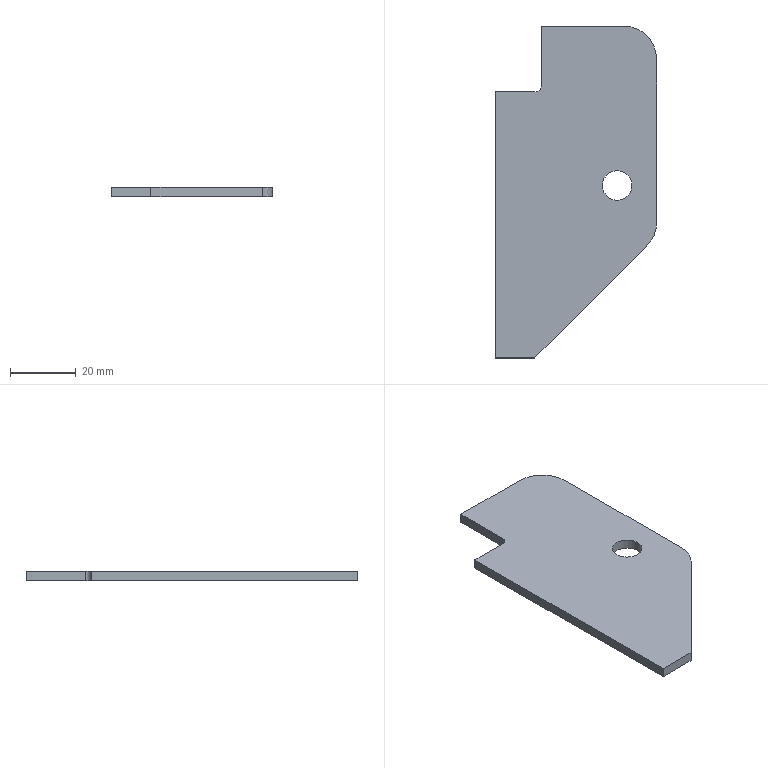Part | STEP file | 750038332 | 1 solid | 14 faces | box 49 x 101 x 3 mm | volume 11694 mm3 | plane 9 | cylinder 5 | commonest cylinder face diameters 9 x2 20 x2 4 x1
STEP:
#1=CARTESIAN_POINT('',(32.5,52.5,3.));
#2=VERTEX_POINT('',#1);
#3=CARTESIAN_POINT('',(41.5,52.5,3.));
#4=VERTEX_POINT('',#3);
#5=CARTESIAN_POINT('',(37.,52.5,3.));
#6=DIRECTION('',(0.,0.,1.));
#7=DIRECTION('',(-1.,0.,0.));
#8=AXIS2_PLACEMENT_3D('',#5,#6,#7);
#9=CIRCLE('',#8,4.5);
#10=EDGE_CURVE('',#2,#4,#9,.T.);
#11=ORIENTED_EDGE('',*,*,#10,.T.);
#12=CARTESIAN_POINT('',(41.5,52.5,0.));
#13=VERTEX_POINT('',#12);
#14=CARTESIAN_POINT('',(41.5,52.5,3.));
#15=DIRECTION('',(0.,0.,-1.));
#16=VECTOR('',#15,1000.);
#17=LINE('',#14,#16);
#18=EDGE_CURVE('',#4,#13,#17,.T.);
#19=ORIENTED_EDGE('',*,*,#18,.T.);
#20=CARTESIAN_POINT('',(32.5,52.5,0.));
#21=VERTEX_POINT('',#20);
#22=CARTESIAN_POINT('',(37.,52.5,0.));
#23=DIRECTION('',(0.,0.,1.));
#24=DIRECTION('',(-1.,0.,0.));
#25=AXIS2_PLACEMENT_3D('',#22,#23,#24);
#26=CIRCLE('',#25,4.5);
#27=EDGE_CURVE('',#21,#13,#26,.T.);
#28=ORIENTED_EDGE('',*,*,#27,.F.);
#29=CARTESIAN_POINT('',(32.5,52.5,3.));
#30=DIRECTION('',(0.,0.,-1.));
#31=VECTOR('',#30,1000.);
#32=LINE('',#29,#31);
#33=EDGE_CURVE('',#2,#21,#32,.T.);
#34=ORIENTED_EDGE('',*,*,#33,.F.);
#35=EDGE_LOOP('',(#11,#19,#28,#34));
#36=FACE_OUTER_BOUND('',#35,.T.);
#37=CARTESIAN_POINT('',(37.,52.5,3.));
#38=DIRECTION('',(0.,0.,-1.));
#39=DIRECTION('',(-1.,0.,0.));
#40=AXIS2_PLACEMENT_3D('',#37,#38,#39);
#41=CYLINDRICAL_SURFACE('',#40,4.5);
#42=ADVANCED_FACE('',(#36),#41,.F.);
#43=ORIENTED_EDGE('',*,*,#10,.F.);
#44=CARTESIAN_POINT('',(37.,52.5,3.));
#45=DIRECTION('',(0.,0.,1.));
#46=DIRECTION('',(-1.,0.,0.));
#47=AXIS2_PLACEMENT_3D('',#44,#45,#46);
#48=CIRCLE('',#47,4.5);
#49=EDGE_CURVE('',#4,#2,#48,.T.);
#50=ORIENTED_EDGE('',*,*,#49,.F.);
#51=EDGE_LOOP('',(#43,#50));
#52=FACE_BOUND('',#51,.T.);
#53=CARTESIAN_POINT('',(39.,101.,3.));
#54=VERTEX_POINT('',#53);
#55=CARTESIAN_POINT('',(49.,91.,3.));
#56=VERTEX_POINT('',#55);
#57=CARTESIAN_POINT('',(39.,91.,3.));
#58=DIRECTION('',(0.,0.,-1.));
#59=DIRECTION('',(-1.,0.,0.));
#60=AXIS2_PLACEMENT_3D('',#57,#58,#59);
#61=CIRCLE('',#60,10.);
#62=EDGE_CURVE('',#54,#56,#61,.T.);
#63=ORIENTED_EDGE('',*,*,#62,.F.);
#64=CARTESIAN_POINT('',(14.,101.,3.));
#65=VERTEX_POINT('',#64);
#66=CARTESIAN_POINT('',(0.,101.,3.));
#67=DIRECTION('',(1.,0.,0.));
#68=VECTOR('',#67,1000.);
#69=LINE('',#66,#68);
#70=EDGE_CURVE('',#65,#54,#69,.T.);
#71=ORIENTED_EDGE('',*,*,#70,.F.);
#72=CARTESIAN_POINT('',(14.,83.,3.));
#73=VERTEX_POINT('',#72);
#74=CARTESIAN_POINT('',(14.,0.,3.));
#75=DIRECTION('',(0.,1.,0.));
#76=VECTOR('',#75,1000.);
#77=LINE('',#74,#76);
#78=EDGE_CURVE('',#73,#65,#77,.T.);
#79=ORIENTED_EDGE('',*,*,#78,.F.);
#80=CARTESIAN_POINT('',(12.,81.,3.));
#81=VERTEX_POINT('',#80);
#82=CARTESIAN_POINT('',(12.,83.,3.));
#83=DIRECTION('',(0.,0.,1.));
#84=DIRECTION('',(1.,0.,0.));
#85=AXIS2_PLACEMENT_3D('',#82,#83,#84);
#86=CIRCLE('',#85,2.);
#87=EDGE_CURVE('',#81,#73,#86,.T.);
#88=ORIENTED_EDGE('',*,*,#87,.F.);
#89=CARTESIAN_POINT('',(0.,81.,3.));
#90=VERTEX_POINT('',#89);
#91=CARTESIAN_POINT('',(0.,81.,3.));
#92=DIRECTION('',(1.,0.,0.));
#93=VECTOR('',#92,1000.);
#94=LINE('',#91,#93);
#95=EDGE_CURVE('',#90,#81,#94,.T.);
#96=ORIENTED_EDGE('',*,*,#95,.F.);
#97=CARTESIAN_POINT('',(0.,0.,3.));
#98=VERTEX_POINT('',#97);
#99=CARTESIAN_POINT('',(0.,0.,3.));
#100=DIRECTION('',(0.,1.,0.));
#101=VECTOR('',#100,1000.);
#102=LINE('',#99,#101);
#103=EDGE_CURVE('',#98,#90,#102,.T.);
#104=ORIENTED_EDGE('',*,*,#103,.F.);
#105=CARTESIAN_POINT('',(12.,0.,3.));
#106=VERTEX_POINT('',#105);
#107=CARTESIAN_POINT('',(0.,0.,3.));
#108=DIRECTION('',(-1.,0.,0.));
#109=VECTOR('',#108,1000.);
#110=LINE('',#107,#109);
#111=EDGE_CURVE('',#106,#98,#110,.T.);
#112=ORIENTED_EDGE('',*,*,#111,.F.);
#113=CARTESIAN_POINT('',(46.071,34.071,3.));
#114=VERTEX_POINT('',#113);
#115=CARTESIAN_POINT('',(46.071,34.071,3.));
#116=DIRECTION('',(-0.7071,-0.7071,0.));
#117=VECTOR('',#116,1000.);
#118=LINE('',#115,#117);
#119=EDGE_CURVE('',#114,#106,#118,.T.);
#120=ORIENTED_EDGE('',*,*,#119,.F.);
#121=CARTESIAN_POINT('',(49.,41.142,3.));
#122=VERTEX_POINT('',#121);
#123=CARTESIAN_POINT('',(39.,41.142,3.));
#124=DIRECTION('',(0.,0.,-1.));
#125=DIRECTION('',(-1.,0.,0.));
#126=AXIS2_PLACEMENT_3D('',#123,#124,#125);
#127=CIRCLE('',#126,10.);
#128=EDGE_CURVE('',#122,#114,#127,.T.);
#129=ORIENTED_EDGE('',*,*,#128,.F.);
#130=CARTESIAN_POINT('',(49.,0.,3.));
#131=DIRECTION('',(0.,-1.,0.));
#132=VECTOR('',#131,1000.);
#133=LINE('',#130,#132);
#134=EDGE_CURVE('',#56,#122,#133,.T.);
#135=ORIENTED_EDGE('',*,*,#134,.F.);
#136=EDGE_LOOP('',(#63,#71,#79,#88,#96,#104,#112,#120,#129,#135));
#137=FACE_OUTER_BOUND('',#136,.T.);
#138=CARTESIAN_POINT('',(0.,0.,3.));
#139=DIRECTION('',(0.,0.,-1.));
#140=DIRECTION('',(-1.,0.,0.));
#141=AXIS2_PLACEMENT_3D('',#138,#139,#140);
#142=PLANE('',#141);
#143=ADVANCED_FACE('',(#52,#137),#142,.F.);
#144=ORIENTED_EDGE('',*,*,#18,.F.);
#145=ORIENTED_EDGE('',*,*,#49,.T.);
#146=ORIENTED_EDGE('',*,*,#33,.T.);
#147=CARTESIAN_POINT('',(37.,52.5,0.));
#148=DIRECTION('',(0.,0.,1.));
#149=DIRECTION('',(-1.,0.,0.));
#150=AXIS2_PLACEMENT_3D('',#147,#148,#149);
#151=CIRCLE('',#150,4.5);
#152=EDGE_CURVE('',#13,#21,#151,.T.);
#153=ORIENTED_EDGE('',*,*,#152,.F.);
#154=EDGE_LOOP('',(#144,#145,#146,#153));
#155=FACE_OUTER_BOUND('',#154,.T.);
#156=CARTESIAN_POINT('',(37.,52.5,3.));
#157=DIRECTION('',(0.,0.,-1.));
#158=DIRECTION('',(-1.,0.,0.));
#159=AXIS2_PLACEMENT_3D('',#156,#157,#158);
#160=CYLINDRICAL_SURFACE('',#159,4.5);
#161=ADVANCED_FACE('',(#155),#160,.F.);
#162=ORIENTED_EDGE('',*,*,#134,.T.);
#163=CARTESIAN_POINT('',(49.,41.142,0.));
#164=VERTEX_POINT('',#163);
#165=CARTESIAN_POINT('',(49.,41.142,3.));
#166=DIRECTION('',(0.,0.,-1.));
#167=VECTOR('',#166,1000.);
#168=LINE('',#165,#167);
#169=EDGE_CURVE('',#122,#164,#168,.T.);
#170=ORIENTED_EDGE('',*,*,#169,.T.);
#171=CARTESIAN_POINT('',(49.,91.,0.));
#172=VERTEX_POINT('',#171);
#173=CARTESIAN_POINT('',(49.,101.,0.));
#174=DIRECTION('',(0.,1.,0.));
#175=VECTOR('',#174,1000.);
#176=LINE('',#173,#175);
#177=EDGE_CURVE('',#164,#172,#176,.T.);
#178=ORIENTED_EDGE('',*,*,#177,.T.);
#179=CARTESIAN_POINT('',(49.,91.,3.));
#180=DIRECTION('',(0.,0.,1.));
#181=VECTOR('',#180,1000.);
#182=LINE('',#179,#181);
#183=EDGE_CURVE('',#172,#56,#182,.T.);
#184=ORIENTED_EDGE('',*,*,#183,.T.);
#185=EDGE_LOOP('',(#162,#170,#178,#184));
#186=FACE_OUTER_BOUND('',#185,.T.);
#187=CARTESIAN_POINT('',(49.,101.,3.));
#188=DIRECTION('',(1.,0.,0.));
#189=DIRECTION('',(0.,1.,0.));
#190=AXIS2_PLACEMENT_3D('',#187,#188,#189);
#191=PLANE('',#190);
#192=ADVANCED_FACE('',(#186),#191,.T.);
#193=CARTESIAN_POINT('',(39.,101.,0.));
#194=VERTEX_POINT('',#193);
#195=CARTESIAN_POINT('',(39.,91.,0.));
#196=DIRECTION('',(0.,0.,1.));
#197=DIRECTION('',(-1.,0.,0.));
#198=AXIS2_PLACEMENT_3D('',#195,#196,#197);
#199=CIRCLE('',#198,10.);
#200=EDGE_CURVE('',#172,#194,#199,.T.);
#201=ORIENTED_EDGE('',*,*,#200,.T.);
#202=CARTESIAN_POINT('',(39.,101.,3.));
#203=DIRECTION('',(0.,0.,1.));
#204=VECTOR('',#203,1000.);
#205=LINE('',#202,#204);
#206=EDGE_CURVE('',#194,#54,#205,.T.);
#207=ORIENTED_EDGE('',*,*,#206,.T.);
#208=ORIENTED_EDGE('',*,*,#62,.T.);
#209=ORIENTED_EDGE('',*,*,#183,.F.);
#210=EDGE_LOOP('',(#201,#207,#208,#209));
#211=FACE_OUTER_BOUND('',#210,.T.);
#212=CARTESIAN_POINT('',(39.,91.,3.));
#213=DIRECTION('',(0.,0.,-1.));
#214=DIRECTION('',(-1.,0.,0.));
#215=AXIS2_PLACEMENT_3D('',#212,#213,#214);
#216=CYLINDRICAL_SURFACE('',#215,10.);
#217=ADVANCED_FACE('',(#211),#216,.T.);
#218=CARTESIAN_POINT('',(14.,101.,0.));
#219=VERTEX_POINT('',#218);
#220=CARTESIAN_POINT('',(14.,101.,0.));
#221=DIRECTION('',(-1.,0.,0.));
#222=VECTOR('',#221,1000.);
#223=LINE('',#220,#222);
#224=EDGE_CURVE('',#194,#219,#223,.T.);
#225=ORIENTED_EDGE('',*,*,#224,.T.);
#226=CARTESIAN_POINT('',(14.,101.,3.));
#227=DIRECTION('',(0.,0.,1.));
#228=VECTOR('',#227,1000.);
#229=LINE('',#226,#228);
#230=EDGE_CURVE('',#219,#65,#229,.T.);
#231=ORIENTED_EDGE('',*,*,#230,.T.);
#232=ORIENTED_EDGE('',*,*,#70,.T.);
#233=ORIENTED_EDGE('',*,*,#206,.F.);
#234=EDGE_LOOP('',(#225,#231,#232,#233));
#235=FACE_OUTER_BOUND('',#234,.T.);
#236=CARTESIAN_POINT('',(14.,101.,3.));
#237=DIRECTION('',(0.,1.,0.));
#238=DIRECTION('',(0.,0.,1.));
#239=AXIS2_PLACEMENT_3D('',#236,#237,#238);
#240=PLANE('',#239);
#241=ADVANCED_FACE('',(#235),#240,.T.);
#242=ORIENTED_EDGE('',*,*,#78,.T.);
#243=ORIENTED_EDGE('',*,*,#230,.F.);
#244=CARTESIAN_POINT('',(14.,83.,0.));
#245=VERTEX_POINT('',#244);
#246=CARTESIAN_POINT('',(14.,81.,0.));
#247=DIRECTION('',(0.,-1.,0.));
#248=VECTOR('',#247,1000.);
#249=LINE('',#246,#248);
#250=EDGE_CURVE('',#219,#245,#249,.T.);
#251=ORIENTED_EDGE('',*,*,#250,.T.);
#252=CARTESIAN_POINT('',(14.,83.,3.));
#253=DIRECTION('',(0.,0.,1.));
#254=VECTOR('',#253,1000.);
#255=LINE('',#252,#254);
#256=EDGE_CURVE('',#245,#73,#255,.T.);
#257=ORIENTED_EDGE('',*,*,#256,.T.);
#258=EDGE_LOOP('',(#242,#243,#251,#257));
#259=FACE_OUTER_BOUND('',#258,.T.);
#260=CARTESIAN_POINT('',(14.,81.,3.));
#261=DIRECTION('',(-1.,0.,0.));
#262=DIRECTION('',(0.,-1.,0.));
#263=AXIS2_PLACEMENT_3D('',#260,#261,#262);
#264=PLANE('',#263);
#265=ADVANCED_FACE('',(#259),#264,.T.);
#266=ORIENTED_EDGE('',*,*,#256,.F.);
#267=CARTESIAN_POINT('',(12.,81.,0.));
#268=VERTEX_POINT('',#267);
#269=CARTESIAN_POINT('',(12.,83.,0.));
#270=DIRECTION('',(0.,0.,1.));
#271=DIRECTION('',(1.,0.,0.));
#272=AXIS2_PLACEMENT_3D('',#269,#270,#271);
#273=CIRCLE('',#272,2.);
#274=EDGE_CURVE('',#268,#245,#273,.T.);
#275=ORIENTED_EDGE('',*,*,#274,.F.);
#276=CARTESIAN_POINT('',(12.,81.,3.));
#277=DIRECTION('',(0.,0.,-1.));
#278=VECTOR('',#277,1000.);
#279=LINE('',#276,#278);
#280=EDGE_CURVE('',#81,#268,#279,.T.);
#281=ORIENTED_EDGE('',*,*,#280,.F.);
#282=ORIENTED_EDGE('',*,*,#87,.T.);
#283=EDGE_LOOP('',(#266,#275,#281,#282));
#284=FACE_OUTER_BOUND('',#283,.T.);
#285=CARTESIAN_POINT('',(12.,83.,3.));
#286=DIRECTION('',(0.,0.,1.));
#287=DIRECTION('',(1.,0.,0.));
#288=AXIS2_PLACEMENT_3D('',#285,#286,#287);
#289=CYLINDRICAL_SURFACE('',#288,2.);
#290=ADVANCED_FACE('',(#284),#289,.F.);
#291=CARTESIAN_POINT('',(0.,81.,0.));
#292=VERTEX_POINT('',#291);
#293=CARTESIAN_POINT('',(0.,81.,0.));
#294=DIRECTION('',(-1.,0.,0.));
#295=VECTOR('',#294,1000.);
#296=LINE('',#293,#295);
#297=EDGE_CURVE('',#268,#292,#296,.T.);
#298=ORIENTED_EDGE('',*,*,#297,.T.);
#299=CARTESIAN_POINT('',(0.,81.,3.));
#300=DIRECTION('',(0.,0.,1.));
#301=VECTOR('',#300,1000.);
#302=LINE('',#299,#301);
#303=EDGE_CURVE('',#292,#90,#302,.T.);
#304=ORIENTED_EDGE('',*,*,#303,.T.);
#305=ORIENTED_EDGE('',*,*,#95,.T.);
#306=ORIENTED_EDGE('',*,*,#280,.T.);
#307=EDGE_LOOP('',(#298,#304,#305,#306));
#308=FACE_OUTER_BOUND('',#307,.T.);
#309=CARTESIAN_POINT('',(0.,81.,3.));
#310=DIRECTION('',(0.,1.,0.));
#311=DIRECTION('',(0.,0.,1.));
#312=AXIS2_PLACEMENT_3D('',#309,#310,#311);
#313=PLANE('',#312);
#314=ADVANCED_FACE('',(#308),#313,.T.);
#315=ORIENTED_EDGE('',*,*,#103,.T.);
#316=ORIENTED_EDGE('',*,*,#303,.F.);
#317=CARTESIAN_POINT('',(0.,0.,0.));
#318=VERTEX_POINT('',#317);
#319=CARTESIAN_POINT('',(0.,0.,0.));
#320=DIRECTION('',(0.,-1.,0.));
#321=VECTOR('',#320,1000.);
#322=LINE('',#319,#321);
#323=EDGE_CURVE('',#292,#318,#322,.T.);
#324=ORIENTED_EDGE('',*,*,#323,.T.);
#325=CARTESIAN_POINT('',(0.,0.,3.));
#326=DIRECTION('',(0.,0.,1.));
#327=VECTOR('',#326,1000.);
#328=LINE('',#325,#327);
#329=EDGE_CURVE('',#318,#98,#328,.T.);
#330=ORIENTED_EDGE('',*,*,#329,.T.);
#331=EDGE_LOOP('',(#315,#316,#324,#330));
#332=FACE_OUTER_BOUND('',#331,.T.);
#333=CARTESIAN_POINT('',(0.,0.,3.));
#334=DIRECTION('',(-1.,0.,0.));
#335=DIRECTION('',(0.,0.,1.));
#336=AXIS2_PLACEMENT_3D('',#333,#334,#335);
#337=PLANE('',#336);
#338=ADVANCED_FACE('',(#332),#337,.T.);
#339=ORIENTED_EDGE('',*,*,#111,.T.);
#340=ORIENTED_EDGE('',*,*,#329,.F.);
#341=CARTESIAN_POINT('',(12.,0.,0.));
#342=VERTEX_POINT('',#341);
#343=CARTESIAN_POINT('',(12.,0.,0.));
#344=DIRECTION('',(1.,0.,0.));
#345=VECTOR('',#344,1000.);
#346=LINE('',#343,#345);
#347=EDGE_CURVE('',#318,#342,#346,.T.);
#348=ORIENTED_EDGE('',*,*,#347,.T.);
#349=CARTESIAN_POINT('',(12.,0.,3.));
#350=DIRECTION('',(0.,0.,1.));
#351=VECTOR('',#350,1000.);
#352=LINE('',#349,#351);
#353=EDGE_CURVE('',#342,#106,#352,.T.);
#354=ORIENTED_EDGE('',*,*,#353,.T.);
#355=EDGE_LOOP('',(#339,#340,#348,#354));
#356=FACE_OUTER_BOUND('',#355,.T.);
#357=CARTESIAN_POINT('',(12.,0.,3.));
#358=DIRECTION('',(0.,-1.,0.));
#359=DIRECTION('',(0.,0.,-1.));
#360=AXIS2_PLACEMENT_3D('',#357,#358,#359);
#361=PLANE('',#360);
#362=ADVANCED_FACE('',(#356),#361,.T.);
#363=ORIENTED_EDGE('',*,*,#119,.T.);
#364=ORIENTED_EDGE('',*,*,#353,.F.);
#365=CARTESIAN_POINT('',(46.071,34.071,0.));
#366=VERTEX_POINT('',#365);
#367=CARTESIAN_POINT('',(49.,37.,0.));
#368=DIRECTION('',(0.7071,0.7071,0.));
#369=VECTOR('',#368,1000.);
#370=LINE('',#367,#369);
#371=EDGE_CURVE('',#342,#366,#370,.T.);
#372=ORIENTED_EDGE('',*,*,#371,.T.);
#373=CARTESIAN_POINT('',(46.071,34.071,3.));
#374=DIRECTION('',(0.,0.,1.));
#375=VECTOR('',#374,1000.);
#376=LINE('',#373,#375);
#377=EDGE_CURVE('',#366,#114,#376,.T.);
#378=ORIENTED_EDGE('',*,*,#377,.T.);
#379=EDGE_LOOP('',(#363,#364,#372,#378));
#380=FACE_OUTER_BOUND('',#379,.T.);
#381=CARTESIAN_POINT('',(49.,37.,3.));
#382=DIRECTION('',(0.7071,-0.7071,0.));
#383=DIRECTION('',(0.7071,0.7071,0.));
#384=AXIS2_PLACEMENT_3D('',#381,#382,#383);
#385=PLANE('',#384);
#386=ADVANCED_FACE('',(#380),#385,.T.);
#387=CARTESIAN_POINT('',(39.,41.142,0.));
#388=DIRECTION('',(0.,0.,1.));
#389=DIRECTION('',(-1.,0.,0.));
#390=AXIS2_PLACEMENT_3D('',#387,#388,#389);
#391=CIRCLE('',#390,10.);
#392=EDGE_CURVE('',#366,#164,#391,.T.);
#393=ORIENTED_EDGE('',*,*,#392,.T.);
#394=ORIENTED_EDGE('',*,*,#169,.F.);
#395=ORIENTED_EDGE('',*,*,#128,.T.);
#396=ORIENTED_EDGE('',*,*,#377,.F.);
#397=EDGE_LOOP('',(#393,#394,#395,#396));
#398=FACE_OUTER_BOUND('',#397,.T.);
#399=CARTESIAN_POINT('',(39.,41.142,3.));
#400=DIRECTION('',(0.,0.,-1.));
#401=DIRECTION('',(-1.,0.,0.));
#402=AXIS2_PLACEMENT_3D('',#399,#400,#401);
#403=CYLINDRICAL_SURFACE('',#402,10.);
#404=ADVANCED_FACE('',(#398),#403,.T.);
#405=ORIENTED_EDGE('',*,*,#27,.T.);
#406=ORIENTED_EDGE('',*,*,#152,.T.);
#407=EDGE_LOOP('',(#405,#406));
#408=FACE_BOUND('',#407,.T.);
#409=ORIENTED_EDGE('',*,*,#274,.T.);
#410=ORIENTED_EDGE('',*,*,#250,.F.);
#411=ORIENTED_EDGE('',*,*,#224,.F.);
#412=ORIENTED_EDGE('',*,*,#200,.F.);
#413=ORIENTED_EDGE('',*,*,#177,.F.);
#414=ORIENTED_EDGE('',*,*,#392,.F.);
#415=ORIENTED_EDGE('',*,*,#371,.F.);
#416=ORIENTED_EDGE('',*,*,#347,.F.);
#417=ORIENTED_EDGE('',*,*,#323,.F.);
#418=ORIENTED_EDGE('',*,*,#297,.F.);
#419=EDGE_LOOP('',(#409,#410,#411,#412,#413,#414,#415,#416,#417,#418));
#420=FACE_OUTER_BOUND('',#419,.T.);
#421=CARTESIAN_POINT('',(0.,0.,0.));
#422=DIRECTION('',(0.,0.,-1.));
#423=DIRECTION('',(-1.,0.,0.));
#424=AXIS2_PLACEMENT_3D('',#421,#422,#423);
#425=PLANE('',#424);
#426=ADVANCED_FACE('',(#408,#420),#425,.T.);
#427=CLOSED_SHELL('',(#42,#143,#161,#192,#217,#241,#265,#290,#314,#338,#362,#386,#404,#426));
#428=MANIFOLD_SOLID_BREP('',#427);
#429=CARTESIAN_POINT('',(0.,0.,0.));
#430=DIRECTION('',(0.,0.,1.));
#431=DIRECTION('',(1.,0.,0.));
#432=AXIS2_PLACEMENT_3D('',#429,#430,#431);
#433=(LENGTH_UNIT()NAMED_UNIT(*)SI_UNIT(.MILLI.,.METRE.));
#434=UNCERTAINTY_MEASURE_WITH_UNIT(LENGTH_MEASURE(0.00001),#433,'','');
#435=(NAMED_UNIT(*)PLANE_ANGLE_UNIT()SI_UNIT($,.RADIAN.));
#436=(NAMED_UNIT(*)SI_UNIT($,.STERADIAN.)SOLID_ANGLE_UNIT());
#437=(GEOMETRIC_REPRESENTATION_CONTEXT(3)GLOBAL_UNCERTAINTY_ASSIGNED_CONTEXT((#434))GLOBAL_UNIT_ASSIGNED_CONTEXT((#433,#435,#436))REPRESENTATION_CONTEXT('',''));
#438=ADVANCED_BREP_SHAPE_REPRESENTATION('',(#428,#432),#437);